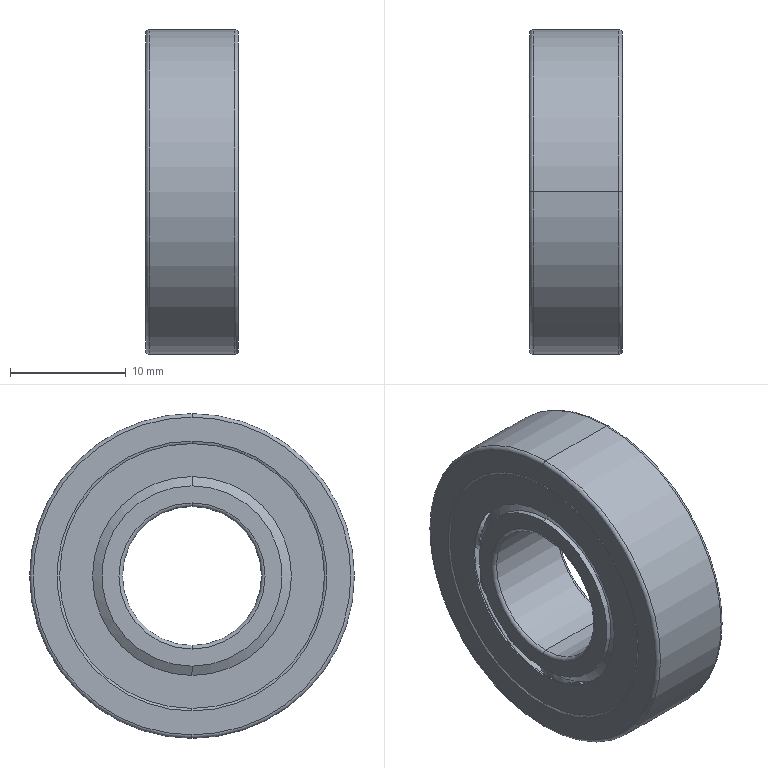Part | SolidWorks | features BaseBody 15 | 15 solids | 234 faces | box 8 x 28 x 28 mm | volume 3006 mm3 | sphere 108 | cylinder 66 | plane 34 | torus 22 | cone 4 | commonest cylinder face diameters 19.2 x25 20.8 x25 15.556 x4 17.333 x4 22.667 x4 12 x2